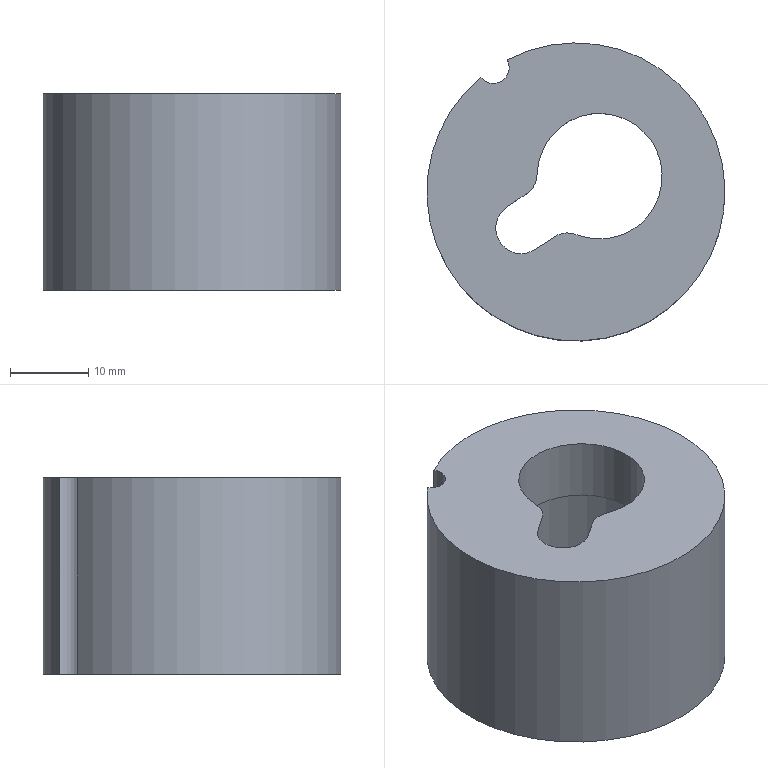Part | NX | features solid 2 | 1 solid | 7 faces | box 38 x 38 x 25 mm | volume 16777 mm3 | plane 3 | cylinder 3 | spline 1 | commonest cylinder face diameters 4 x1 26.6 x1 38 x1